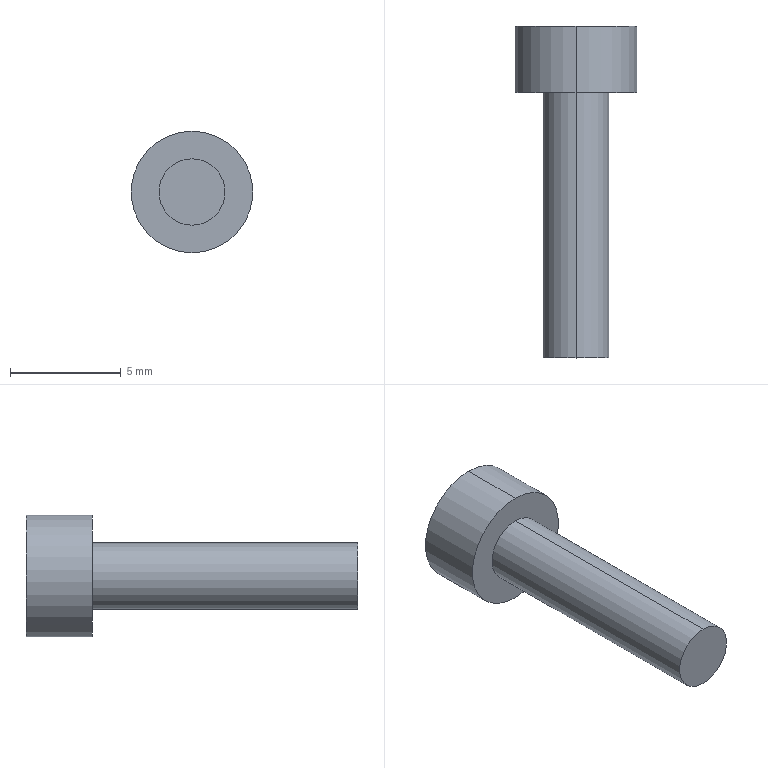Part | STEP file | NEZI-R_E-LMPJC30L35-14-15-LK5 | 1 solid | 14 faces | box 5.5 x 15 x 5.5 mm | volume 148.72 mm3 | plane 10 | cylinder 4 | commonest cylinder face diameters 3 x2 5.5 x2
STEP:
#1=CARTESIAN_POINT('',(0.,0.,0.));
#2=DIRECTION('',(0.,0.,1.));
#3=DIRECTION('',(1.,0.,0.));
#4=AXIS2_PLACEMENT_3D('',#1,#2,#3);
#5=CARTESIAN_POINT('',(0.,-12.,-1.5));
#6=VERTEX_POINT('',#5);
#7=CARTESIAN_POINT('',(0.,-12.,1.5));
#8=VERTEX_POINT('',#7);
#9=CARTESIAN_POINT('',(0.,-12.,0.));
#10=DIRECTION('',(0.,-1.,0.));
#11=DIRECTION('',(0.,0.,-1.));
#12=AXIS2_PLACEMENT_3D('',#9,#10,#11);
#13=CIRCLE('',#12,1.5);
#14=CARTESIAN_POINT('',(0.,-12.,0.));
#15=DIRECTION('',(0.,1.,0.));
#16=DIRECTION('',(0.,0.,1.));
#17=AXIS2_PLACEMENT_3D('',#14,#15,#16);
#18=CYLINDRICAL_SURFACE('',#17,1.5);
#19=CARTESIAN_POINT('',(3.142,0.));
#20=DIRECTION('',(-1.,0.));
#21=VECTOR('',#20,1.);
#22=LINE('',#19,#21);
#23=(GEOMETRIC_REPRESENTATION_CONTEXT(2)PARAMETRIC_REPRESENTATION_CONTEXT()REPRESENTATION_CONTEXT('',''));
#24=DEFINITIONAL_REPRESENTATION('',(#22),#23);
#25=PCURVE('',#18,#24);
#26=CARTESIAN_POINT('',(0.,-12.,0.));
#27=DIRECTION('',(0.,-1.,0.));
#28=DIRECTION('',(0.,0.,-1.));
#29=AXIS2_PLACEMENT_3D('',#26,#27,#28);
#30=PLANE('',#29);
#31=CARTESIAN_POINT('',(0.,0.));
#32=DIRECTION('',(1.,0.));
#33=AXIS2_PLACEMENT_2D('',#31,#32);
#34=CIRCLE('',#33,1.5);
#35=(GEOMETRIC_REPRESENTATION_CONTEXT(2)PARAMETRIC_REPRESENTATION_CONTEXT()REPRESENTATION_CONTEXT('',''));
#36=DEFINITIONAL_REPRESENTATION('',(#34),#35);
#37=PCURVE('',#30,#36);
#38=SURFACE_CURVE('',#13,(#25,#37),.PCURVE_S1.);
#39=EDGE_CURVE('',#6,#8,#38,.T.);
#40=ORIENTED_EDGE('',*,*,#39,.F.);
#41=CARTESIAN_POINT('',(0.,0.,-1.5));
#42=VERTEX_POINT('',#41);
#43=CARTESIAN_POINT('',(0.,-12.,-1.5));
#44=DIRECTION('',(0.,1.,0.));
#45=VECTOR('',#44,1.);
#46=LINE('',#43,#45);
#47=CARTESIAN_POINT('',(3.142,0.));
#48=DIRECTION('',(0.,1.));
#49=VECTOR('',#48,1.);
#50=LINE('',#47,#49);
#51=(GEOMETRIC_REPRESENTATION_CONTEXT(2)PARAMETRIC_REPRESENTATION_CONTEXT()REPRESENTATION_CONTEXT('',''));
#52=DEFINITIONAL_REPRESENTATION('',(#50),#51);
#53=PCURVE('',#18,#52);
#54=CARTESIAN_POINT('',(0.,-12.,0.));
#55=DIRECTION('',(0.,1.,0.));
#56=DIRECTION('',(0.,0.,1.));
#57=AXIS2_PLACEMENT_3D('',#54,#55,#56);
#58=CYLINDRICAL_SURFACE('',#57,1.5);
#59=CARTESIAN_POINT('',(3.142,0.));
#60=DIRECTION('',(0.,1.));
#61=VECTOR('',#60,1.);
#62=LINE('',#59,#61);
#63=(GEOMETRIC_REPRESENTATION_CONTEXT(2)PARAMETRIC_REPRESENTATION_CONTEXT()REPRESENTATION_CONTEXT('',''));
#64=DEFINITIONAL_REPRESENTATION('',(#62),#63);
#65=PCURVE('',#58,#64);
#66=SURFACE_CURVE('',#46,(#53,#65),.PCURVE_S1.);
#67=EDGE_CURVE('',#6,#42,#66,.T.);
#68=ORIENTED_EDGE('',*,*,#67,.T.);
#69=CARTESIAN_POINT('',(0.,0.,1.5));
#70=VERTEX_POINT('',#69);
#71=CARTESIAN_POINT('',(0.,0.,0.));
#72=DIRECTION('',(0.,-1.,0.));
#73=DIRECTION('',(0.,0.,1.));
#74=AXIS2_PLACEMENT_3D('',#71,#72,#73);
#75=CIRCLE('',#74,1.5);
#76=CARTESIAN_POINT('',(6.283,12.));
#77=DIRECTION('',(-1.,0.));
#78=VECTOR('',#77,1.);
#79=LINE('',#76,#78);
#80=(GEOMETRIC_REPRESENTATION_CONTEXT(2)PARAMETRIC_REPRESENTATION_CONTEXT()REPRESENTATION_CONTEXT('',''));
#81=DEFINITIONAL_REPRESENTATION('',(#79),#80);
#82=PCURVE('',#18,#81);
#83=CARTESIAN_POINT('',(0.,0.,0.));
#84=DIRECTION('',(0.,1.,0.));
#85=DIRECTION('',(0.,0.,1.));
#86=AXIS2_PLACEMENT_3D('',#83,#84,#85);
#87=PLANE('',#86);
#88=CARTESIAN_POINT('',(1.5,0.));
#89=CARTESIAN_POINT('',(1.5,-2.598));
#90=CARTESIAN_POINT('',(-0.75,-1.299));
#91=CARTESIAN_POINT('',(-3.,0.));
#92=CARTESIAN_POINT('',(-0.75,1.299));
#93=CARTESIAN_POINT('',(1.5,2.598));
#94=CARTESIAN_POINT('',(1.5,0.));
#95=(BOUNDED_CURVE()B_SPLINE_CURVE(2,(#88,#89,#90,#91,#92,#93,#94),.UNSPECIFIED.,.T.,.F.)B_SPLINE_CURVE_WITH_KNOTS((1,2,2,2,2,1),(-2.094,0.,2.094,4.189,6.283,8.378),.UNSPECIFIED.)CURVE()GEOMETRIC_REPRESENTATION_ITEM()RATIONAL_B_SPLINE_CURVE((1.,0.5,1.,0.5,1.,0.5,1.))REPRESENTATION_ITEM(''));
#96=(GEOMETRIC_REPRESENTATION_CONTEXT(2)PARAMETRIC_REPRESENTATION_CONTEXT()REPRESENTATION_CONTEXT('',''));
#97=DEFINITIONAL_REPRESENTATION('',(#95),#96);
#98=PCURVE('',#87,#97);
#99=SURFACE_CURVE('',#75,(#82,#98),.PCURVE_S1.);
#100=EDGE_CURVE('',#42,#70,#99,.T.);
#101=ORIENTED_EDGE('',*,*,#100,.T.);
#102=CARTESIAN_POINT('',(0.,-12.,1.5));
#103=DIRECTION('',(0.,1.,0.));
#104=VECTOR('',#103,1.);
#105=LINE('',#102,#104);
#106=CARTESIAN_POINT('',(0.,0.));
#107=DIRECTION('',(0.,1.));
#108=VECTOR('',#107,1.);
#109=LINE('',#106,#108);
#110=(GEOMETRIC_REPRESENTATION_CONTEXT(2)PARAMETRIC_REPRESENTATION_CONTEXT()REPRESENTATION_CONTEXT('',''));
#111=DEFINITIONAL_REPRESENTATION('',(#109),#110);
#112=PCURVE('',#18,#111);
#113=CARTESIAN_POINT('',(6.283,0.));
#114=DIRECTION('',(0.,1.));
#115=VECTOR('',#114,1.);
#116=LINE('',#113,#115);
#117=(GEOMETRIC_REPRESENTATION_CONTEXT(2)PARAMETRIC_REPRESENTATION_CONTEXT()REPRESENTATION_CONTEXT('',''));
#118=DEFINITIONAL_REPRESENTATION('',(#116),#117);
#119=PCURVE('',#58,#118);
#120=SURFACE_CURVE('',#105,(#112,#119),.PCURVE_S1.);
#121=EDGE_CURVE('',#8,#70,#120,.T.);
#122=ORIENTED_EDGE('',*,*,#121,.F.);
#123=EDGE_LOOP('',(#40,#68,#101,#122));
#124=FACE_BOUND('',#123,.T.);
#125=ADVANCED_FACE('',(#124),#18,.T.);
#126=CARTESIAN_POINT('',(0.,3.,2.75));
#127=VERTEX_POINT('',#126);
#128=CARTESIAN_POINT('',(0.,3.,-2.75));
#129=VERTEX_POINT('',#128);
#130=CARTESIAN_POINT('',(0.,3.,0.));
#131=DIRECTION('',(0.,1.,0.));
#132=DIRECTION('',(0.,0.,1.));
#133=AXIS2_PLACEMENT_3D('',#130,#131,#132);
#134=CIRCLE('',#133,2.75);
#135=CARTESIAN_POINT('',(0.,3.,0.));
#136=DIRECTION('',(0.,-1.,0.));
#137=DIRECTION('',(0.,0.,-1.));
#138=AXIS2_PLACEMENT_3D('',#135,#136,#137);
#139=CYLINDRICAL_SURFACE('',#138,2.75);
#140=CARTESIAN_POINT('',(3.142,0.));
#141=DIRECTION('',(-1.,0.));
#142=VECTOR('',#141,1.);
#143=LINE('',#140,#142);
#144=(GEOMETRIC_REPRESENTATION_CONTEXT(2)PARAMETRIC_REPRESENTATION_CONTEXT()REPRESENTATION_CONTEXT('',''));
#145=DEFINITIONAL_REPRESENTATION('',(#143),#144);
#146=PCURVE('',#139,#145);
#147=CARTESIAN_POINT('',(0.,3.,0.));
#148=DIRECTION('',(0.,1.,0.));
#149=DIRECTION('',(0.,0.,1.));
#150=AXIS2_PLACEMENT_3D('',#147,#148,#149);
#151=PLANE('',#150);
#152=CARTESIAN_POINT('',(0.,0.));
#153=DIRECTION('',(1.,0.));
#154=AXIS2_PLACEMENT_2D('',#152,#153);
#155=CIRCLE('',#154,2.75);
#156=(GEOMETRIC_REPRESENTATION_CONTEXT(2)PARAMETRIC_REPRESENTATION_CONTEXT()REPRESENTATION_CONTEXT('',''));
#157=DEFINITIONAL_REPRESENTATION('',(#155),#156);
#158=PCURVE('',#151,#157);
#159=SURFACE_CURVE('',#134,(#146,#158),.PCURVE_S1.);
#160=EDGE_CURVE('',#127,#129,#159,.T.);
#161=ORIENTED_EDGE('',*,*,#160,.F.);
#162=CARTESIAN_POINT('',(0.,0.,2.75));
#163=VERTEX_POINT('',#162);
#164=CARTESIAN_POINT('',(0.,3.,2.75));
#165=DIRECTION('',(0.,-1.,0.));
#166=VECTOR('',#165,1.);
#167=LINE('',#164,#166);
#168=CARTESIAN_POINT('',(3.142,0.));
#169=DIRECTION('',(0.,1.));
#170=VECTOR('',#169,1.);
#171=LINE('',#168,#170);
#172=(GEOMETRIC_REPRESENTATION_CONTEXT(2)PARAMETRIC_REPRESENTATION_CONTEXT()REPRESENTATION_CONTEXT('',''));
#173=DEFINITIONAL_REPRESENTATION('',(#171),#172);
#174=PCURVE('',#139,#173);
#175=CARTESIAN_POINT('',(0.,3.,0.));
#176=DIRECTION('',(0.,-1.,0.));
#177=DIRECTION('',(0.,0.,-1.));
#178=AXIS2_PLACEMENT_3D('',#175,#176,#177);
#179=CYLINDRICAL_SURFACE('',#178,2.75);
#180=CARTESIAN_POINT('',(3.142,0.));
#181=DIRECTION('',(0.,1.));
#182=VECTOR('',#181,1.);
#183=LINE('',#180,#182);
#184=(GEOMETRIC_REPRESENTATION_CONTEXT(2)PARAMETRIC_REPRESENTATION_CONTEXT()REPRESENTATION_CONTEXT('',''));
#185=DEFINITIONAL_REPRESENTATION('',(#183),#184);
#186=PCURVE('',#179,#185);
#187=SURFACE_CURVE('',#167,(#174,#186),.PCURVE_S1.);
#188=EDGE_CURVE('',#127,#163,#187,.T.);
#189=ORIENTED_EDGE('',*,*,#188,.T.);
#190=CARTESIAN_POINT('',(0.,0.,-2.75));
#191=VERTEX_POINT('',#190);
#192=CARTESIAN_POINT('',(0.,0.,0.));
#193=DIRECTION('',(0.,1.,0.));
#194=DIRECTION('',(0.,0.,1.));
#195=AXIS2_PLACEMENT_3D('',#192,#193,#194);
#196=CIRCLE('',#195,2.75);
#197=CARTESIAN_POINT('',(3.142,3.));
#198=DIRECTION('',(-1.,0.));
#199=VECTOR('',#198,1.);
#200=LINE('',#197,#199);
#201=(GEOMETRIC_REPRESENTATION_CONTEXT(2)PARAMETRIC_REPRESENTATION_CONTEXT()REPRESENTATION_CONTEXT('',''));
#202=DEFINITIONAL_REPRESENTATION('',(#200),#201);
#203=PCURVE('',#139,#202);
#204=CARTESIAN_POINT('',(0.,0.));
#205=DIRECTION('',(1.,0.));
#206=AXIS2_PLACEMENT_2D('',#204,#205);
#207=CIRCLE('',#206,2.75);
#208=(GEOMETRIC_REPRESENTATION_CONTEXT(2)PARAMETRIC_REPRESENTATION_CONTEXT()REPRESENTATION_CONTEXT('',''));
#209=DEFINITIONAL_REPRESENTATION('',(#207),#208);
#210=PCURVE('',#87,#209);
#211=SURFACE_CURVE('',#196,(#203,#210),.PCURVE_S1.);
#212=EDGE_CURVE('',#163,#191,#211,.T.);
#213=ORIENTED_EDGE('',*,*,#212,.T.);
#214=CARTESIAN_POINT('',(0.,3.,-2.75));
#215=DIRECTION('',(0.,-1.,0.));
#216=VECTOR('',#215,1.);
#217=LINE('',#214,#216);
#218=CARTESIAN_POINT('',(0.,0.));
#219=DIRECTION('',(0.,1.));
#220=VECTOR('',#219,1.);
#221=LINE('',#218,#220);
#222=(GEOMETRIC_REPRESENTATION_CONTEXT(2)PARAMETRIC_REPRESENTATION_CONTEXT()REPRESENTATION_CONTEXT('',''));
#223=DEFINITIONAL_REPRESENTATION('',(#221),#222);
#224=PCURVE('',#139,#223);
#225=CARTESIAN_POINT('',(6.283,0.));
#226=DIRECTION('',(0.,1.));
#227=VECTOR('',#226,1.);
#228=LINE('',#225,#227);
#229=(GEOMETRIC_REPRESENTATION_CONTEXT(2)PARAMETRIC_REPRESENTATION_CONTEXT()REPRESENTATION_CONTEXT('',''));
#230=DEFINITIONAL_REPRESENTATION('',(#228),#229);
#231=PCURVE('',#179,#230);
#232=SURFACE_CURVE('',#217,(#224,#231),.PCURVE_S1.);
#233=EDGE_CURVE('',#129,#191,#232,.T.);
#234=ORIENTED_EDGE('',*,*,#233,.F.);
#235=EDGE_LOOP('',(#161,#189,#213,#234));
#236=FACE_BOUND('',#235,.T.);
#237=ADVANCED_FACE('',(#236),#139,.T.);
#238=ORIENTED_EDGE('',*,*,#188,.F.);
#239=CARTESIAN_POINT('',(0.,3.,0.));
#240=DIRECTION('',(0.,1.,0.));
#241=DIRECTION('',(0.,0.,1.));
#242=AXIS2_PLACEMENT_3D('',#239,#240,#241);
#243=CIRCLE('',#242,2.75);
#244=CARTESIAN_POINT('',(9.425,0.));
#245=DIRECTION('',(-1.,0.));
#246=VECTOR('',#245,1.);
#247=LINE('',#244,#246);
#248=(GEOMETRIC_REPRESENTATION_CONTEXT(2)PARAMETRIC_REPRESENTATION_CONTEXT()REPRESENTATION_CONTEXT('',''));
#249=DEFINITIONAL_REPRESENTATION('',(#247),#248);
#250=PCURVE('',#179,#249);
#251=CARTESIAN_POINT('',(0.,0.));
#252=DIRECTION('',(1.,0.));
#253=AXIS2_PLACEMENT_2D('',#251,#252);
#254=CIRCLE('',#253,2.75);
#255=(GEOMETRIC_REPRESENTATION_CONTEXT(2)PARAMETRIC_REPRESENTATION_CONTEXT()REPRESENTATION_CONTEXT('',''));
#256=DEFINITIONAL_REPRESENTATION('',(#254),#255);
#257=PCURVE('',#151,#256);
#258=SURFACE_CURVE('',#243,(#250,#257),.PCURVE_S1.);
#259=EDGE_CURVE('',#129,#127,#258,.T.);
#260=ORIENTED_EDGE('',*,*,#259,.F.);
#261=ORIENTED_EDGE('',*,*,#233,.T.);
#262=CARTESIAN_POINT('',(0.,0.,0.));
#263=DIRECTION('',(0.,1.,0.));
#264=DIRECTION('',(0.,0.,1.));
#265=AXIS2_PLACEMENT_3D('',#262,#263,#264);
#266=CIRCLE('',#265,2.75);
#267=CARTESIAN_POINT('',(9.425,3.));
#268=DIRECTION('',(-1.,0.));
#269=VECTOR('',#268,1.);
#270=LINE('',#267,#269);
#271=(GEOMETRIC_REPRESENTATION_CONTEXT(2)PARAMETRIC_REPRESENTATION_CONTEXT()REPRESENTATION_CONTEXT('',''));
#272=DEFINITIONAL_REPRESENTATION('',(#270),#271);
#273=PCURVE('',#179,#272);
#274=CARTESIAN_POINT('',(0.,0.));
#275=DIRECTION('',(1.,0.));
#276=AXIS2_PLACEMENT_2D('',#274,#275);
#277=CIRCLE('',#276,2.75);
#278=(GEOMETRIC_REPRESENTATION_CONTEXT(2)PARAMETRIC_REPRESENTATION_CONTEXT()REPRESENTATION_CONTEXT('',''));
#279=DEFINITIONAL_REPRESENTATION('',(#277),#278);
#280=PCURVE('',#87,#279);
#281=SURFACE_CURVE('',#266,(#273,#280),.PCURVE_S1.);
#282=EDGE_CURVE('',#191,#163,#281,.T.);
#283=ORIENTED_EDGE('',*,*,#282,.T.);
#284=EDGE_LOOP('',(#238,#260,#261,#283));
#285=FACE_BOUND('',#284,.T.);
#286=ADVANCED_FACE('',(#285),#179,.T.);
#287=CARTESIAN_POINT('',(1.28,3.,-0.739));
#288=VERTEX_POINT('',#287);
#289=CARTESIAN_POINT('',(0.,3.,-1.478));
#290=VERTEX_POINT('',#289);
#291=CARTESIAN_POINT('',(1.28,3.,-0.739));
#292=DIRECTION('',(-0.866,0.,-0.5));
#293=VECTOR('',#292,1.);
#294=LINE('',#291,#293);
#295=CARTESIAN_POINT('',(-0.739,1.28));
#296=DIRECTION('',(-0.5,-0.866));
#297=VECTOR('',#296,1.);
#298=LINE('',#295,#297);
#299=(GEOMETRIC_REPRESENTATION_CONTEXT(2)PARAMETRIC_REPRESENTATION_CONTEXT()REPRESENTATION_CONTEXT('',''));
#300=DEFINITIONAL_REPRESENTATION('',(#298),#299);
#301=PCURVE('',#151,#300);
#302=CARTESIAN_POINT('',(1.28,1.7,-0.739));
#303=DIRECTION('',(0.5,0.,-0.866));
#304=DIRECTION('',(-0.866,0.,-0.5));
#305=AXIS2_PLACEMENT_3D('',#302,#303,#304);
#306=PLANE('',#305);
#307=CARTESIAN_POINT('',(0.,1.3));
#308=DIRECTION('',(1.,0.));
#309=VECTOR('',#308,1.);
#310=LINE('',#307,#309);
#311=(GEOMETRIC_REPRESENTATION_CONTEXT(2)PARAMETRIC_REPRESENTATION_CONTEXT()REPRESENTATION_CONTEXT('',''));
#312=DEFINITIONAL_REPRESENTATION('',(#310),#311);
#313=PCURVE('',#306,#312);
#314=SURFACE_CURVE('',#294,(#301,#313),.PCURVE_S1.);
#315=EDGE_CURVE('',#288,#290,#314,.T.);
#316=ORIENTED_EDGE('',*,*,#315,.F.);
#317=CARTESIAN_POINT('',(1.28,3.,0.739));
#318=VERTEX_POINT('',#317);
#319=CARTESIAN_POINT('',(1.28,3.,0.739));
#320=DIRECTION('',(0.,0.,-1.));
#321=VECTOR('',#320,1.);
#322=LINE('',#319,#321);
#323=CARTESIAN_POINT('',(0.739,1.28));
#324=DIRECTION('',(-1.,0.));
#325=VECTOR('',#324,1.);
#326=LINE('',#323,#325);
#327=(GEOMETRIC_REPRESENTATION_CONTEXT(2)PARAMETRIC_REPRESENTATION_CONTEXT()REPRESENTATION_CONTEXT('',''));
#328=DEFINITIONAL_REPRESENTATION('',(#326),#327);
#329=PCURVE('',#151,#328);
#330=CARTESIAN_POINT('',(1.28,1.7,0.739));
#331=DIRECTION('',(1.,0.,0.));
#332=DIRECTION('',(0.,0.,-1.));
#333=AXIS2_PLACEMENT_3D('',#330,#331,#332);
#334=PLANE('',#333);
#335=CARTESIAN_POINT('',(0.,1.3));
#336=DIRECTION('',(1.,0.));
#337=VECTOR('',#336,1.);
#338=LINE('',#335,#337);
#339=(GEOMETRIC_REPRESENTATION_CONTEXT(2)PARAMETRIC_REPRESENTATION_CONTEXT()REPRESENTATION_CONTEXT('',''));
#340=DEFINITIONAL_REPRESENTATION('',(#338),#339);
#341=PCURVE('',#334,#340);
#342=SURFACE_CURVE('',#322,(#329,#341),.PCURVE_S1.);
#343=EDGE_CURVE('',#318,#288,#342,.T.);
#344=ORIENTED_EDGE('',*,*,#343,.F.);
#345=CARTESIAN_POINT('',(0.,3.,1.478));
#346=VERTEX_POINT('',#345);
#347=CARTESIAN_POINT('',(0.,3.,1.478));
#348=DIRECTION('',(0.866,0.,-0.5));
#349=VECTOR('',#348,1.);
#350=LINE('',#347,#349);
#351=CARTESIAN_POINT('',(1.478,0.));
#352=DIRECTION('',(-0.5,0.866));
#353=VECTOR('',#352,1.);
#354=LINE('',#351,#353);
#355=(GEOMETRIC_REPRESENTATION_CONTEXT(2)PARAMETRIC_REPRESENTATION_CONTEXT()REPRESENTATION_CONTEXT('',''));
#356=DEFINITIONAL_REPRESENTATION('',(#354),#355);
#357=PCURVE('',#151,#356);
#358=CARTESIAN_POINT('',(0.,1.7,1.478));
#359=DIRECTION('',(0.5,0.,0.866));
#360=DIRECTION('',(0.866,0.,-0.5));
#361=AXIS2_PLACEMENT_3D('',#358,#359,#360);
#362=PLANE('',#361);
#363=CARTESIAN_POINT('',(0.,1.3));
#364=DIRECTION('',(1.,0.));
#365=VECTOR('',#364,1.);
#366=LINE('',#363,#365);
#367=(GEOMETRIC_REPRESENTATION_CONTEXT(2)PARAMETRIC_REPRESENTATION_CONTEXT()REPRESENTATION_CONTEXT('',''));
#368=DEFINITIONAL_REPRESENTATION('',(#366),#367);
#369=PCURVE('',#362,#368);
#370=SURFACE_CURVE('',#350,(#357,#369),.PCURVE_S1.);
#371=EDGE_CURVE('',#346,#318,#370,.T.);
#372=ORIENTED_EDGE('',*,*,#371,.F.);
#373=CARTESIAN_POINT('',(-1.28,3.,0.739));
#374=VERTEX_POINT('',#373);
#375=CARTESIAN_POINT('',(-1.28,3.,0.739));
#376=DIRECTION('',(0.866,0.,0.5));
#377=VECTOR('',#376,1.);
#378=LINE('',#375,#377);
#379=CARTESIAN_POINT('',(0.739,-1.28));
#380=DIRECTION('',(0.5,0.866));
#381=VECTOR('',#380,1.);
#382=LINE('',#379,#381);
#383=(GEOMETRIC_REPRESENTATION_CONTEXT(2)PARAMETRIC_REPRESENTATION_CONTEXT()REPRESENTATION_CONTEXT('',''));
#384=DEFINITIONAL_REPRESENTATION('',(#382),#383);
#385=PCURVE('',#151,#384);
#386=CARTESIAN_POINT('',(-1.28,1.7,0.739));
#387=DIRECTION('',(-0.5,0.,0.866));
#388=DIRECTION('',(0.866,0.,0.5));
#389=AXIS2_PLACEMENT_3D('',#386,#387,#388);
#390=PLANE('',#389);
#391=CARTESIAN_POINT('',(0.,1.3));
#392=DIRECTION('',(1.,0.));
#393=VECTOR('',#392,1.);
#394=LINE('',#391,#393);
#395=(GEOMETRIC_REPRESENTATION_CONTEXT(2)PARAMETRIC_REPRESENTATION_CONTEXT()REPRESENTATION_CONTEXT('',''));
#396=DEFINITIONAL_REPRESENTATION('',(#394),#395);
#397=PCURVE('',#390,#396);
#398=SURFACE_CURVE('',#378,(#385,#397),.PCURVE_S1.);
#399=EDGE_CURVE('',#374,#346,#398,.T.);
#400=ORIENTED_EDGE('',*,*,#399,.F.);
#401=CARTESIAN_POINT('',(-1.28,3.,-0.739));
#402=VERTEX_POINT('',#401);
#403=CARTESIAN_POINT('',(-1.28,3.,-0.739));
#404=DIRECTION('',(0.,0.,1.));
#405=VECTOR('',#404,1.);
#406=LINE('',#403,#405);
#407=CARTESIAN_POINT('',(-0.739,-1.28));
#408=DIRECTION('',(1.,0.));
#409=VECTOR('',#408,1.);
#410=LINE('',#407,#409);
#411=(GEOMETRIC_REPRESENTATION_CONTEXT(2)PARAMETRIC_REPRESENTATION_CONTEXT()REPRESENTATION_CONTEXT('',''));
#412=DEFINITIONAL_REPRESENTATION('',(#410),#411);
#413=PCURVE('',#151,#412);
#414=CARTESIAN_POINT('',(-1.28,1.7,-0.739));
#415=DIRECTION('',(-1.,0.,0.));
#416=DIRECTION('',(0.,0.,1.));
#417=AXIS2_PLACEMENT_3D('',#414,#415,#416);
#418=PLANE('',#417);
#419=CARTESIAN_POINT('',(0.,1.3));
#420=DIRECTION('',(1.,0.));
#421=VECTOR('',#420,1.);
#422=LINE('',#419,#421);
#423=(GEOMETRIC_REPRESENTATION_CONTEXT(2)PARAMETRIC_REPRESENTATION_CONTEXT()REPRESENTATION_CONTEXT('',''));
#424=DEFINITIONAL_REPRESENTATION('',(#422),#423);
#425=PCURVE('',#418,#424);
#426=SURFACE_CURVE('',#406,(#413,#425),.PCURVE_S1.);
#427=EDGE_CURVE('',#402,#374,#426,.T.);
#428=ORIENTED_EDGE('',*,*,#427,.F.);
#429=CARTESIAN_POINT('',(0.,3.,-1.478));
#430=DIRECTION('',(-0.866,0.,0.5));
#431=VECTOR('',#430,1.);
#432=LINE('',#429,#431);
#433=CARTESIAN_POINT('',(-1.478,0.));
#434=DIRECTION('',(0.5,-0.866));
#435=VECTOR('',#434,1.);
#436=LINE('',#433,#435);
#437=(GEOMETRIC_REPRESENTATION_CONTEXT(2)PARAMETRIC_REPRESENTATION_CONTEXT()REPRESENTATION_CONTEXT('',''));
#438=DEFINITIONAL_REPRESENTATION('',(#436),#437);
#439=PCURVE('',#151,#438);
#440=CARTESIAN_POINT('',(0.,1.7,-1.478));
#441=DIRECTION('',(-0.5,0.,-0.866));
#442=DIRECTION('',(-0.866,0.,0.5));
#443=AXIS2_PLACEMENT_3D('',#440,#441,#442);
#444=PLANE('',#443);
#445=CARTESIAN_POINT('',(0.,1.3));
#446=DIRECTION('',(1.,0.));
#447=VECTOR('',#446,1.);
#448=LINE('',#445,#447);
#449=(GEOMETRIC_REPRESENTATION_CONTEXT(2)PARAMETRIC_REPRESENTATION_CONTEXT()REPRESENTATION_CONTEXT('',''));
#450=DEFINITIONAL_REPRESENTATION('',(#448),#449);
#451=PCURVE('',#444,#450);
#452=SURFACE_CURVE('',#432,(#439,#451),.PCURVE_S1.);
#453=EDGE_CURVE('',#290,#402,#452,.T.);
#454=ORIENTED_EDGE('',*,*,#453,.F.);
#455=EDGE_LOOP('',(#316,#344,#372,#400,#428,#454));
#456=FACE_BOUND('',#455,.T.);
#457=ORIENTED_EDGE('',*,*,#259,.T.);
#458=ORIENTED_EDGE('',*,*,#160,.T.);
#459=EDGE_LOOP('',(#457,#458));
#460=FACE_BOUND('',#459,.T.);
#461=ADVANCED_FACE('',(#456,#460),#151,.T.);
#462=CARTESIAN_POINT('',(0.,0.,0.));
#463=DIRECTION('',(0.,-1.,0.));
#464=DIRECTION('',(0.,0.,1.));
#465=AXIS2_PLACEMENT_3D('',#462,#463,#464);
#466=CIRCLE('',#465,1.5);
#467=CARTESIAN_POINT('',(1.5,0.));
#468=CARTESIAN_POINT('',(1.5,-2.598));
#469=CARTESIAN_POINT('',(-0.75,-1.299));
#470=CARTESIAN_POINT('',(-3.,0.));
#471=CARTESIAN_POINT('',(-0.75,1.299));
#472=CARTESIAN_POINT('',(1.5,2.598));
#473=CARTESIAN_POINT('',(1.5,0.));
#474=(BOUNDED_CURVE()B_SPLINE_CURVE(2,(#467,#468,#469,#470,#471,#472,#473),.UNSPECIFIED.,.T.,.F.)B_SPLINE_CURVE_WITH_KNOTS((1,2,2,2,2,1),(-2.094,0.,2.094,4.189,6.283,8.378),.UNSPECIFIED.)CURVE()GEOMETRIC_REPRESENTATION_ITEM()RATIONAL_B_SPLINE_CURVE((1.,0.5,1.,0.5,1.,0.5,1.))REPRESENTATION_ITEM(''));
#475=(GEOMETRIC_REPRESENTATION_CONTEXT(2)PARAMETRIC_REPRESENTATION_CONTEXT()REPRESENTATION_CONTEXT('',''));
#476=DEFINITIONAL_REPRESENTATION('',(#474),#475);
#477=PCURVE('',#87,#476);
#478=CARTESIAN_POINT('',(6.283,12.));
#479=DIRECTION('',(-1.,0.));
#480=VECTOR('',#479,1.);
#481=LINE('',#478,#480);
#482=(GEOMETRIC_REPRESENTATION_CONTEXT(2)PARAMETRIC_REPRESENTATION_CONTEXT()REPRESENTATION_CONTEXT('',''));
#483=DEFINITIONAL_REPRESENTATION('',(#481),#482);
#484=PCURVE('',#58,#483);
#485=SURFACE_CURVE('',#466,(#477,#484),.PCURVE_S1.);
#486=EDGE_CURVE('',#70,#42,#485,.T.);
#487=ORIENTED_EDGE('',*,*,#486,.F.);
#488=ORIENTED_EDGE('',*,*,#100,.F.);
#489=EDGE_LOOP('',(#487,#488));
#490=FACE_BOUND('',#489,.T.);
#491=ORIENTED_EDGE('',*,*,#282,.F.);
#492=ORIENTED_EDGE('',*,*,#212,.F.);
#493=EDGE_LOOP('',(#491,#492));
#494=FACE_BOUND('',#493,.T.);
#495=ADVANCED_FACE('',(#490,#494),#87,.F.);
#496=ORIENTED_EDGE('',*,*,#67,.F.);
#497=CARTESIAN_POINT('',(0.,-12.,0.));
#498=DIRECTION('',(0.,-1.,0.));
#499=DIRECTION('',(0.,0.,-1.));
#500=AXIS2_PLACEMENT_3D('',#497,#498,#499);
#501=CIRCLE('',#500,1.5);
#502=CARTESIAN_POINT('',(9.425,0.));
#503=DIRECTION('',(-1.,0.));
#504=VECTOR('',#503,1.);
#505=LINE('',#502,#504);
#506=(GEOMETRIC_REPRESENTATION_CONTEXT(2)PARAMETRIC_REPRESENTATION_CONTEXT()REPRESENTATION_CONTEXT('',''));
#507=DEFINITIONAL_REPRESENTATION('',(#505),#506);
#508=PCURVE('',#58,#507);
#509=CARTESIAN_POINT('',(0.,0.));
#510=DIRECTION('',(1.,0.));
#511=AXIS2_PLACEMENT_2D('',#509,#510);
#512=CIRCLE('',#511,1.5);
#513=(GEOMETRIC_REPRESENTATION_CONTEXT(2)PARAMETRIC_REPRESENTATION_CONTEXT()REPRESENTATION_CONTEXT('',''));
#514=DEFINITIONAL_REPRESENTATION('',(#512),#513);
#515=PCURVE('',#30,#514);
#516=SURFACE_CURVE('',#501,(#508,#515),.PCURVE_S1.);
#517=EDGE_CURVE('',#8,#6,#516,.T.);
#518=ORIENTED_EDGE('',*,*,#517,.F.);
#519=ORIENTED_EDGE('',*,*,#121,.T.);
#520=ORIENTED_EDGE('',*,*,#486,.T.);
#521=EDGE_LOOP('',(#496,#518,#519,#520));
#522=FACE_BOUND('',#521,.T.);
#523=ADVANCED_FACE('',(#522),#58,.T.);
#524=ORIENTED_EDGE('',*,*,#517,.T.);
#525=ORIENTED_EDGE('',*,*,#39,.T.);
#526=EDGE_LOOP('',(#524,#525));
#527=FACE_BOUND('',#526,.T.);
#528=ADVANCED_FACE('',(#527),#30,.T.);
#529=ORIENTED_EDGE('',*,*,#315,.T.);
#530=CARTESIAN_POINT('',(0.,1.7,-1.478));
#531=VERTEX_POINT('',#530);
#532=CARTESIAN_POINT('',(0.,1.7,-1.478));
#533=DIRECTION('',(0.,1.,0.));
#534=VECTOR('',#533,1.);
#535=LINE('',#532,#534);
#536=CARTESIAN_POINT('',(1.478,0.));
#537=DIRECTION('',(0.,1.));
#538=VECTOR('',#537,1.);
#539=LINE('',#536,#538);
#540=(GEOMETRIC_REPRESENTATION_CONTEXT(2)PARAMETRIC_REPRESENTATION_CONTEXT()REPRESENTATION_CONTEXT('',''));
#541=DEFINITIONAL_REPRESENTATION('',(#539),#540);
#542=PCURVE('',#306,#541);
#543=CARTESIAN_POINT('',(0.,0.));
#544=DIRECTION('',(0.,1.));
#545=VECTOR('',#544,1.);
#546=LINE('',#543,#545);
#547=(GEOMETRIC_REPRESENTATION_CONTEXT(2)PARAMETRIC_REPRESENTATION_CONTEXT()REPRESENTATION_CONTEXT('',''));
#548=DEFINITIONAL_REPRESENTATION('',(#546),#547);
#549=PCURVE('',#444,#548);
#550=SURFACE_CURVE('',#535,(#542,#549),.PCURVE_S1.);
#551=EDGE_CURVE('',#531,#290,#550,.T.);
#552=ORIENTED_EDGE('',*,*,#551,.F.);
#553=CARTESIAN_POINT('',(1.28,1.7,-0.739));
#554=VERTEX_POINT('',#553);
#555=CARTESIAN_POINT('',(1.28,1.7,-0.739));
#556=DIRECTION('',(-0.866,0.,-0.5));
#557=VECTOR('',#556,1.);
#558=LINE('',#555,#557);
#559=CARTESIAN_POINT('',(0.,0.));
#560=DIRECTION('',(1.,0.));
#561=VECTOR('',#560,1.);
#562=LINE('',#559,#561);
#563=(GEOMETRIC_REPRESENTATION_CONTEXT(2)PARAMETRIC_REPRESENTATION_CONTEXT()REPRESENTATION_CONTEXT('',''));
#564=DEFINITIONAL_REPRESENTATION('',(#562),#563);
#565=PCURVE('',#306,#564);
#566=CARTESIAN_POINT('',(0.,1.7,0.));
#567=DIRECTION('',(0.,1.,0.));
#568=DIRECTION('',(0.,0.,1.));
#569=AXIS2_PLACEMENT_3D('',#566,#567,#568);
#570=PLANE('',#569);
#571=CARTESIAN_POINT('',(-0.739,1.28));
#572=DIRECTION('',(-0.5,-0.866));
#573=VECTOR('',#572,1.);
#574=LINE('',#571,#573);
#575=(GEOMETRIC_REPRESENTATION_CONTEXT(2)PARAMETRIC_REPRESENTATION_CONTEXT()REPRESENTATION_CONTEXT('',''));
#576=DEFINITIONAL_REPRESENTATION('',(#574),#575);
#577=PCURVE('',#570,#576);
#578=SURFACE_CURVE('',#558,(#565,#577),.PCURVE_S1.);
#579=EDGE_CURVE('',#554,#531,#578,.T.);
#580=ORIENTED_EDGE('',*,*,#579,.F.);
#581=CARTESIAN_POINT('',(1.28,1.7,-0.739));
#582=DIRECTION('',(0.,1.,0.));
#583=VECTOR('',#582,1.);
#584=LINE('',#581,#583);
#585=CARTESIAN_POINT('',(0.,0.));
#586=DIRECTION('',(0.,1.));
#587=VECTOR('',#586,1.);
#588=LINE('',#585,#587);
#589=(GEOMETRIC_REPRESENTATION_CONTEXT(2)PARAMETRIC_REPRESENTATION_CONTEXT()REPRESENTATION_CONTEXT('',''));
#590=DEFINITIONAL_REPRESENTATION('',(#588),#589);
#591=PCURVE('',#306,#590);
#592=CARTESIAN_POINT('',(1.478,0.));
#593=DIRECTION('',(0.,1.));
#594=VECTOR('',#593,1.);
#595=LINE('',#592,#594);
#596=(GEOMETRIC_REPRESENTATION_CONTEXT(2)PARAMETRIC_REPRESENTATION_CONTEXT()REPRESENTATION_CONTEXT('',''));
#597=DEFINITIONAL_REPRESENTATION('',(#595),#596);
#598=PCURVE('',#334,#597);
#599=SURFACE_CURVE('',#584,(#591,#598),.PCURVE_S1.);
#600=EDGE_CURVE('',#554,#288,#599,.T.);
#601=ORIENTED_EDGE('',*,*,#600,.T.);
#602=EDGE_LOOP('',(#529,#552,#580,#601));
#603=FACE_BOUND('',#602,.T.);
#604=ADVANCED_FACE('',(#603),#306,.F.);
#605=ORIENTED_EDGE('',*,*,#343,.T.);
#606=ORIENTED_EDGE('',*,*,#600,.F.);
#607=CARTESIAN_POINT('',(1.28,1.7,0.739));
#608=VERTEX_POINT('',#607);
#609=CARTESIAN_POINT('',(1.28,1.7,0.739));
#610=DIRECTION('',(0.,0.,-1.));
#611=VECTOR('',#610,1.);
#612=LINE('',#609,#611);
#613=CARTESIAN_POINT('',(0.,0.));
#614=DIRECTION('',(1.,0.));
#615=VECTOR('',#614,1.);
#616=LINE('',#613,#615);
#617=(GEOMETRIC_REPRESENTATION_CONTEXT(2)PARAMETRIC_REPRESENTATION_CONTEXT()REPRESENTATION_CONTEXT('',''));
#618=DEFINITIONAL_REPRESENTATION('',(#616),#617);
#619=PCURVE('',#334,#618);
#620=CARTESIAN_POINT('',(0.739,1.28));
#621=DIRECTION('',(-1.,0.));
#622=VECTOR('',#621,1.);
#623=LINE('',#620,#622);
#624=(GEOMETRIC_REPRESENTATION_CONTEXT(2)PARAMETRIC_REPRESENTATION_CONTEXT()REPRESENTATION_CONTEXT('',''));
#625=DEFINITIONAL_REPRESENTATION('',(#623),#624);
#626=PCURVE('',#570,#625);
#627=SURFACE_CURVE('',#612,(#619,#626),.PCURVE_S1.);
#628=EDGE_CURVE('',#608,#554,#627,.T.);
#629=ORIENTED_EDGE('',*,*,#628,.F.);
#630=CARTESIAN_POINT('',(1.28,1.7,0.739));
#631=DIRECTION('',(0.,1.,0.));
#632=VECTOR('',#631,1.);
#633=LINE('',#630,#632);
#634=CARTESIAN_POINT('',(0.,0.));
#635=DIRECTION('',(0.,1.));
#636=VECTOR('',#635,1.);
#637=LINE('',#634,#636);
#638=(GEOMETRIC_REPRESENTATION_CONTEXT(2)PARAMETRIC_REPRESENTATION_CONTEXT()REPRESENTATION_CONTEXT('',''));
#639=DEFINITIONAL_REPRESENTATION('',(#637),#638);
#640=PCURVE('',#334,#639);
#641=CARTESIAN_POINT('',(1.478,0.));
#642=DIRECTION('',(0.,1.));
#643=VECTOR('',#642,1.);
#644=LINE('',#641,#643);
#645=(GEOMETRIC_REPRESENTATION_CONTEXT(2)PARAMETRIC_REPRESENTATION_CONTEXT()REPRESENTATION_CONTEXT('',''));
#646=DEFINITIONAL_REPRESENTATION('',(#644),#645);
#647=PCURVE('',#362,#646);
#648=SURFACE_CURVE('',#633,(#640,#647),.PCURVE_S1.);
#649=EDGE_CURVE('',#608,#318,#648,.T.);
#650=ORIENTED_EDGE('',*,*,#649,.T.);
#651=EDGE_LOOP('',(#605,#606,#629,#650));
#652=FACE_BOUND('',#651,.T.);
#653=ADVANCED_FACE('',(#652),#334,.F.);
#654=ORIENTED_EDGE('',*,*,#371,.T.);
#655=ORIENTED_EDGE('',*,*,#649,.F.);
#656=CARTESIAN_POINT('',(0.,1.7,1.478));
#657=VERTEX_POINT('',#656);
#658=CARTESIAN_POINT('',(0.,1.7,1.478));
#659=DIRECTION('',(0.866,0.,-0.5));
#660=VECTOR('',#659,1.);
#661=LINE('',#658,#660);
#662=CARTESIAN_POINT('',(0.,0.));
#663=DIRECTION('',(1.,0.));
#664=VECTOR('',#663,1.);
#665=LINE('',#662,#664);
#666=(GEOMETRIC_REPRESENTATION_CONTEXT(2)PARAMETRIC_REPRESENTATION_CONTEXT()REPRESENTATION_CONTEXT('',''));
#667=DEFINITIONAL_REPRESENTATION('',(#665),#666);
#668=PCURVE('',#362,#667);
#669=CARTESIAN_POINT('',(1.478,0.));
#670=DIRECTION('',(-0.5,0.866));
#671=VECTOR('',#670,1.);
#672=LINE('',#669,#671);
#673=(GEOMETRIC_REPRESENTATION_CONTEXT(2)PARAMETRIC_REPRESENTATION_CONTEXT()REPRESENTATION_CONTEXT('',''));
#674=DEFINITIONAL_REPRESENTATION('',(#672),#673);
#675=PCURVE('',#570,#674);
#676=SURFACE_CURVE('',#661,(#668,#675),.PCURVE_S1.);
#677=EDGE_CURVE('',#657,#608,#676,.T.);
#678=ORIENTED_EDGE('',*,*,#677,.F.);
#679=CARTESIAN_POINT('',(0.,1.7,1.478));
#680=DIRECTION('',(0.,1.,0.));
#681=VECTOR('',#680,1.);
#682=LINE('',#679,#681);
#683=CARTESIAN_POINT('',(0.,0.));
#684=DIRECTION('',(0.,1.));
#685=VECTOR('',#684,1.);
#686=LINE('',#683,#685);
#687=(GEOMETRIC_REPRESENTATION_CONTEXT(2)PARAMETRIC_REPRESENTATION_CONTEXT()REPRESENTATION_CONTEXT('',''));
#688=DEFINITIONAL_REPRESENTATION('',(#686),#687);
#689=PCURVE('',#362,#688);
#690=CARTESIAN_POINT('',(1.478,0.));
#691=DIRECTION('',(0.,1.));
#692=VECTOR('',#691,1.);
#693=LINE('',#690,#692);
#694=(GEOMETRIC_REPRESENTATION_CONTEXT(2)PARAMETRIC_REPRESENTATION_CONTEXT()REPRESENTATION_CONTEXT('',''));
#695=DEFINITIONAL_REPRESENTATION('',(#693),#694);
#696=PCURVE('',#390,#695);
#697=SURFACE_CURVE('',#682,(#689,#696),.PCURVE_S1.);
#698=EDGE_CURVE('',#657,#346,#697,.T.);
#699=ORIENTED_EDGE('',*,*,#698,.T.);
#700=EDGE_LOOP('',(#654,#655,#678,#699));
#701=FACE_BOUND('',#700,.T.);
#702=ADVANCED_FACE('',(#701),#362,.F.);
#703=ORIENTED_EDGE('',*,*,#399,.T.);
#704=ORIENTED_EDGE('',*,*,#698,.F.);
#705=CARTESIAN_POINT('',(-1.28,1.7,0.739));
#706=VERTEX_POINT('',#705);
#707=CARTESIAN_POINT('',(-1.28,1.7,0.739));
#708=DIRECTION('',(0.866,0.,0.5));
#709=VECTOR('',#708,1.);
#710=LINE('',#707,#709);
#711=CARTESIAN_POINT('',(0.,0.));
#712=DIRECTION('',(1.,0.));
#713=VECTOR('',#712,1.);
#714=LINE('',#711,#713);
#715=(GEOMETRIC_REPRESENTATION_CONTEXT(2)PARAMETRIC_REPRESENTATION_CONTEXT()REPRESENTATION_CONTEXT('',''));
#716=DEFINITIONAL_REPRESENTATION('',(#714),#715);
#717=PCURVE('',#390,#716);
#718=CARTESIAN_POINT('',(0.739,-1.28));
#719=DIRECTION('',(0.5,0.866));
#720=VECTOR('',#719,1.);
#721=LINE('',#718,#720);
#722=(GEOMETRIC_REPRESENTATION_CONTEXT(2)PARAMETRIC_REPRESENTATION_CONTEXT()REPRESENTATION_CONTEXT('',''));
#723=DEFINITIONAL_REPRESENTATION('',(#721),#722);
#724=PCURVE('',#570,#723);
#725=SURFACE_CURVE('',#710,(#717,#724),.PCURVE_S1.);
#726=EDGE_CURVE('',#706,#657,#725,.T.);
#727=ORIENTED_EDGE('',*,*,#726,.F.);
#728=CARTESIAN_POINT('',(-1.28,1.7,0.739));
#729=DIRECTION('',(0.,1.,0.));
#730=VECTOR('',#729,1.);
#731=LINE('',#728,#730);
#732=CARTESIAN_POINT('',(0.,0.));
#733=DIRECTION('',(0.,1.));
#734=VECTOR('',#733,1.);
#735=LINE('',#732,#734);
#736=(GEOMETRIC_REPRESENTATION_CONTEXT(2)PARAMETRIC_REPRESENTATION_CONTEXT()REPRESENTATION_CONTEXT('',''));
#737=DEFINITIONAL_REPRESENTATION('',(#735),#736);
#738=PCURVE('',#390,#737);
#739=CARTESIAN_POINT('',(1.478,0.));
#740=DIRECTION('',(0.,1.));
#741=VECTOR('',#740,1.);
#742=LINE('',#739,#741);
#743=(GEOMETRIC_REPRESENTATION_CONTEXT(2)PARAMETRIC_REPRESENTATION_CONTEXT()REPRESENTATION_CONTEXT('',''));
#744=DEFINITIONAL_REPRESENTATION('',(#742),#743);
#745=PCURVE('',#418,#744);
#746=SURFACE_CURVE('',#731,(#738,#745),.PCURVE_S1.);
#747=EDGE_CURVE('',#706,#374,#746,.T.);
#748=ORIENTED_EDGE('',*,*,#747,.T.);
#749=EDGE_LOOP('',(#703,#704,#727,#748));
#750=FACE_BOUND('',#749,.T.);
#751=ADVANCED_FACE('',(#750),#390,.F.);
#752=ORIENTED_EDGE('',*,*,#427,.T.);
#753=ORIENTED_EDGE('',*,*,#747,.F.);
#754=CARTESIAN_POINT('',(-1.28,1.7,-0.739));
#755=VERTEX_POINT('',#754);
#756=CARTESIAN_POINT('',(-1.28,1.7,-0.739));
#757=DIRECTION('',(0.,0.,1.));
#758=VECTOR('',#757,1.);
#759=LINE('',#756,#758);
#760=CARTESIAN_POINT('',(0.,0.));
#761=DIRECTION('',(1.,0.));
#762=VECTOR('',#761,1.);
#763=LINE('',#760,#762);
#764=(GEOMETRIC_REPRESENTATION_CONTEXT(2)PARAMETRIC_REPRESENTATION_CONTEXT()REPRESENTATION_CONTEXT('',''));
#765=DEFINITIONAL_REPRESENTATION('',(#763),#764);
#766=PCURVE('',#418,#765);
#767=CARTESIAN_POINT('',(-0.739,-1.28));
#768=DIRECTION('',(1.,0.));
#769=VECTOR('',#768,1.);
#770=LINE('',#767,#769);
#771=(GEOMETRIC_REPRESENTATION_CONTEXT(2)PARAMETRIC_REPRESENTATION_CONTEXT()REPRESENTATION_CONTEXT('',''));
#772=DEFINITIONAL_REPRESENTATION('',(#770),#771);
#773=PCURVE('',#570,#772);
#774=SURFACE_CURVE('',#759,(#766,#773),.PCURVE_S1.);
#775=EDGE_CURVE('',#755,#706,#774,.T.);
#776=ORIENTED_EDGE('',*,*,#775,.F.);
#777=CARTESIAN_POINT('',(-1.28,1.7,-0.739));
#778=DIRECTION('',(0.,1.,0.));
#779=VECTOR('',#778,1.);
#780=LINE('',#777,#779);
#781=CARTESIAN_POINT('',(0.,0.));
#782=DIRECTION('',(0.,1.));
#783=VECTOR('',#782,1.);
#784=LINE('',#781,#783);
#785=(GEOMETRIC_REPRESENTATION_CONTEXT(2)PARAMETRIC_REPRESENTATION_CONTEXT()REPRESENTATION_CONTEXT('',''));
#786=DEFINITIONAL_REPRESENTATION('',(#784),#785);
#787=PCURVE('',#418,#786);
#788=CARTESIAN_POINT('',(1.478,0.));
#789=DIRECTION('',(0.,1.));
#790=VECTOR('',#789,1.);
#791=LINE('',#788,#790);
#792=(GEOMETRIC_REPRESENTATION_CONTEXT(2)PARAMETRIC_REPRESENTATION_CONTEXT()REPRESENTATION_CONTEXT('',''));
#793=DEFINITIONAL_REPRESENTATION('',(#791),#792);
#794=PCURVE('',#444,#793);
#795=SURFACE_CURVE('',#780,(#787,#794),.PCURVE_S1.);
#796=EDGE_CURVE('',#755,#402,#795,.T.);
#797=ORIENTED_EDGE('',*,*,#796,.T.);
#798=EDGE_LOOP('',(#752,#753,#776,#797));
#799=FACE_BOUND('',#798,.T.);
#800=ADVANCED_FACE('',(#799),#418,.F.);
#801=ORIENTED_EDGE('',*,*,#453,.T.);
#802=ORIENTED_EDGE('',*,*,#796,.F.);
#803=CARTESIAN_POINT('',(0.,1.7,-1.478));
#804=DIRECTION('',(-0.866,0.,0.5));
#805=VECTOR('',#804,1.);
#806=LINE('',#803,#805);
#807=CARTESIAN_POINT('',(0.,0.));
#808=DIRECTION('',(1.,0.));
#809=VECTOR('',#808,1.);
#810=LINE('',#807,#809);
#811=(GEOMETRIC_REPRESENTATION_CONTEXT(2)PARAMETRIC_REPRESENTATION_CONTEXT()REPRESENTATION_CONTEXT('',''));
#812=DEFINITIONAL_REPRESENTATION('',(#810),#811);
#813=PCURVE('',#444,#812);
#814=CARTESIAN_POINT('',(-1.478,0.));
#815=DIRECTION('',(0.5,-0.866));
#816=VECTOR('',#815,1.);
#817=LINE('',#814,#816);
#818=(GEOMETRIC_REPRESENTATION_CONTEXT(2)PARAMETRIC_REPRESENTATION_CONTEXT()REPRESENTATION_CONTEXT('',''));
#819=DEFINITIONAL_REPRESENTATION('',(#817),#818);
#820=PCURVE('',#570,#819);
#821=SURFACE_CURVE('',#806,(#813,#820),.PCURVE_S1.);
#822=EDGE_CURVE('',#531,#755,#821,.T.);
#823=ORIENTED_EDGE('',*,*,#822,.F.);
#824=ORIENTED_EDGE('',*,*,#551,.T.);
#825=EDGE_LOOP('',(#801,#802,#823,#824));
#826=FACE_BOUND('',#825,.T.);
#827=ADVANCED_FACE('',(#826),#444,.F.);
#828=ORIENTED_EDGE('',*,*,#579,.T.);
#829=ORIENTED_EDGE('',*,*,#822,.T.);
#830=ORIENTED_EDGE('',*,*,#775,.T.);
#831=ORIENTED_EDGE('',*,*,#726,.T.);
#832=ORIENTED_EDGE('',*,*,#677,.T.);
#833=ORIENTED_EDGE('',*,*,#628,.T.);
#834=EDGE_LOOP('',(#828,#829,#830,#831,#832,#833));
#835=FACE_BOUND('',#834,.T.);
#836=ADVANCED_FACE('',(#835),#570,.T.);
#837=CLOSED_SHELL('',(#125,#237,#286,#461,#495,#523,#528,#604,#653,#702,#751,#800,#827,#836));
#838=MANIFOLD_SOLID_BREP('',#837);
#839=(LENGTH_UNIT()NAMED_UNIT(*)SI_UNIT(.MILLI.,.METRE.));
#840=UNCERTAINTY_MEASURE_WITH_UNIT(LENGTH_MEASURE(0.0000001),#839,'','');
#841=(NAMED_UNIT(*)PLANE_ANGLE_UNIT()SI_UNIT($,.RADIAN.));
#842=(NAMED_UNIT(*)SI_UNIT($,.STERADIAN.)SOLID_ANGLE_UNIT());
#843=(GEOMETRIC_REPRESENTATION_CONTEXT(3)GLOBAL_UNCERTAINTY_ASSIGNED_CONTEXT((#840))GLOBAL_UNIT_ASSIGNED_CONTEXT((#839,#841,#842))REPRESENTATION_CONTEXT('',''));
#844=ADVANCED_BREP_SHAPE_REPRESENTATION('',(#4,#838),#843);